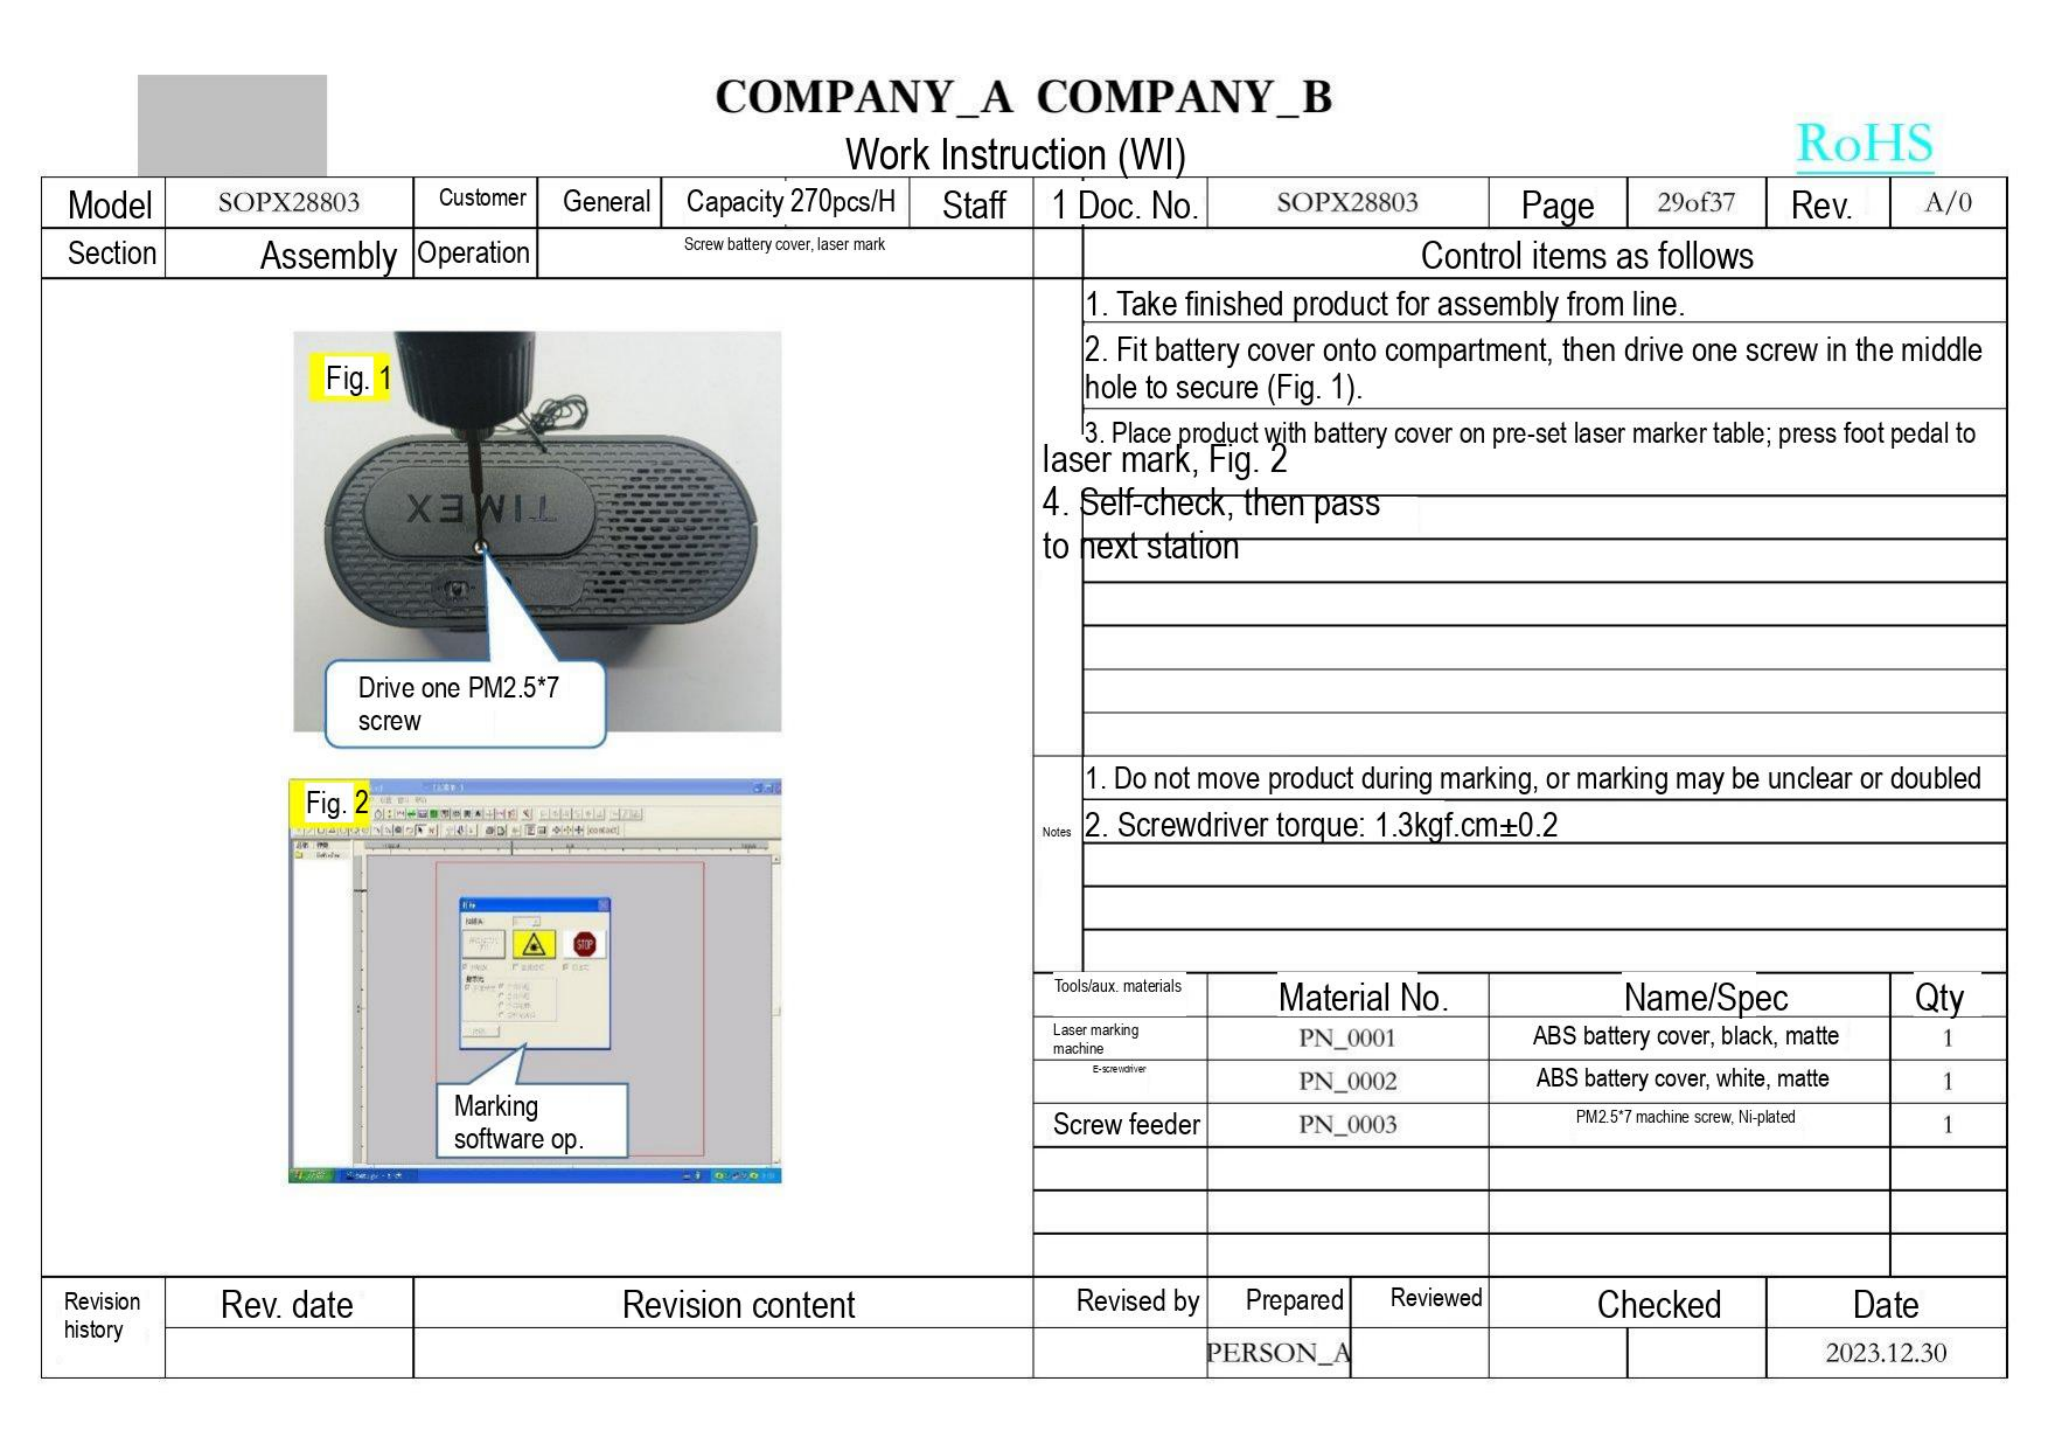# COMPANY_A COMPANY_B
## Work Instruction (WI)
RoHS

| Model | SOPX28803 | Customer | General | Capacity 270pcs/H | Staff | 1 | Doc. No. | SOPX28803 | Page | 29of37 | Rev. | A/0 |
|---|---|---|---|---|---|---|---|---|---|---|---|---|
| Section | Assembly | Operation | Screw battery cover, laser mark | | | | | | | | | |

**Control items as follows**

1. Take finished product for assembly from line.
2. Fit battery cover onto compartment, then drive one screw in the middle hole to secure (Fig. 1).
3. Place product with battery cover on pre-set laser marker table; press foot pedal to laser mark, Fig. 2
4. Self-check, then pass to next station

Fig. 1

Drive one PM2.5*7 screw

Fig. 2

Marking software op.

**Notes**

1. Do not move product during marking, or marking may be unclear or doubled
2. Screwdriver torque: 1.3kgf.cm±0.2

| Tools/aux. materials | Material No. | Name/Spec | Qty |
|---|---|---|---|
| Laser marking machine | PN_0001 | ABS battery cover, black, matte | 1 |
| E-screwdriver | PN_0002 | ABS battery cover, white, matte | 1 |
| Screw feeder | PN_0003 | PM2.5*7 machine screw, Ni-plated | 1 |

| Revision history | Rev. date | Revision content | Revised by | Prepared | Reviewed | Checked | Date |
|---|---|---|---|---|---|---|---|
| | | | | PERSON_A | | | 2023.12.30 |
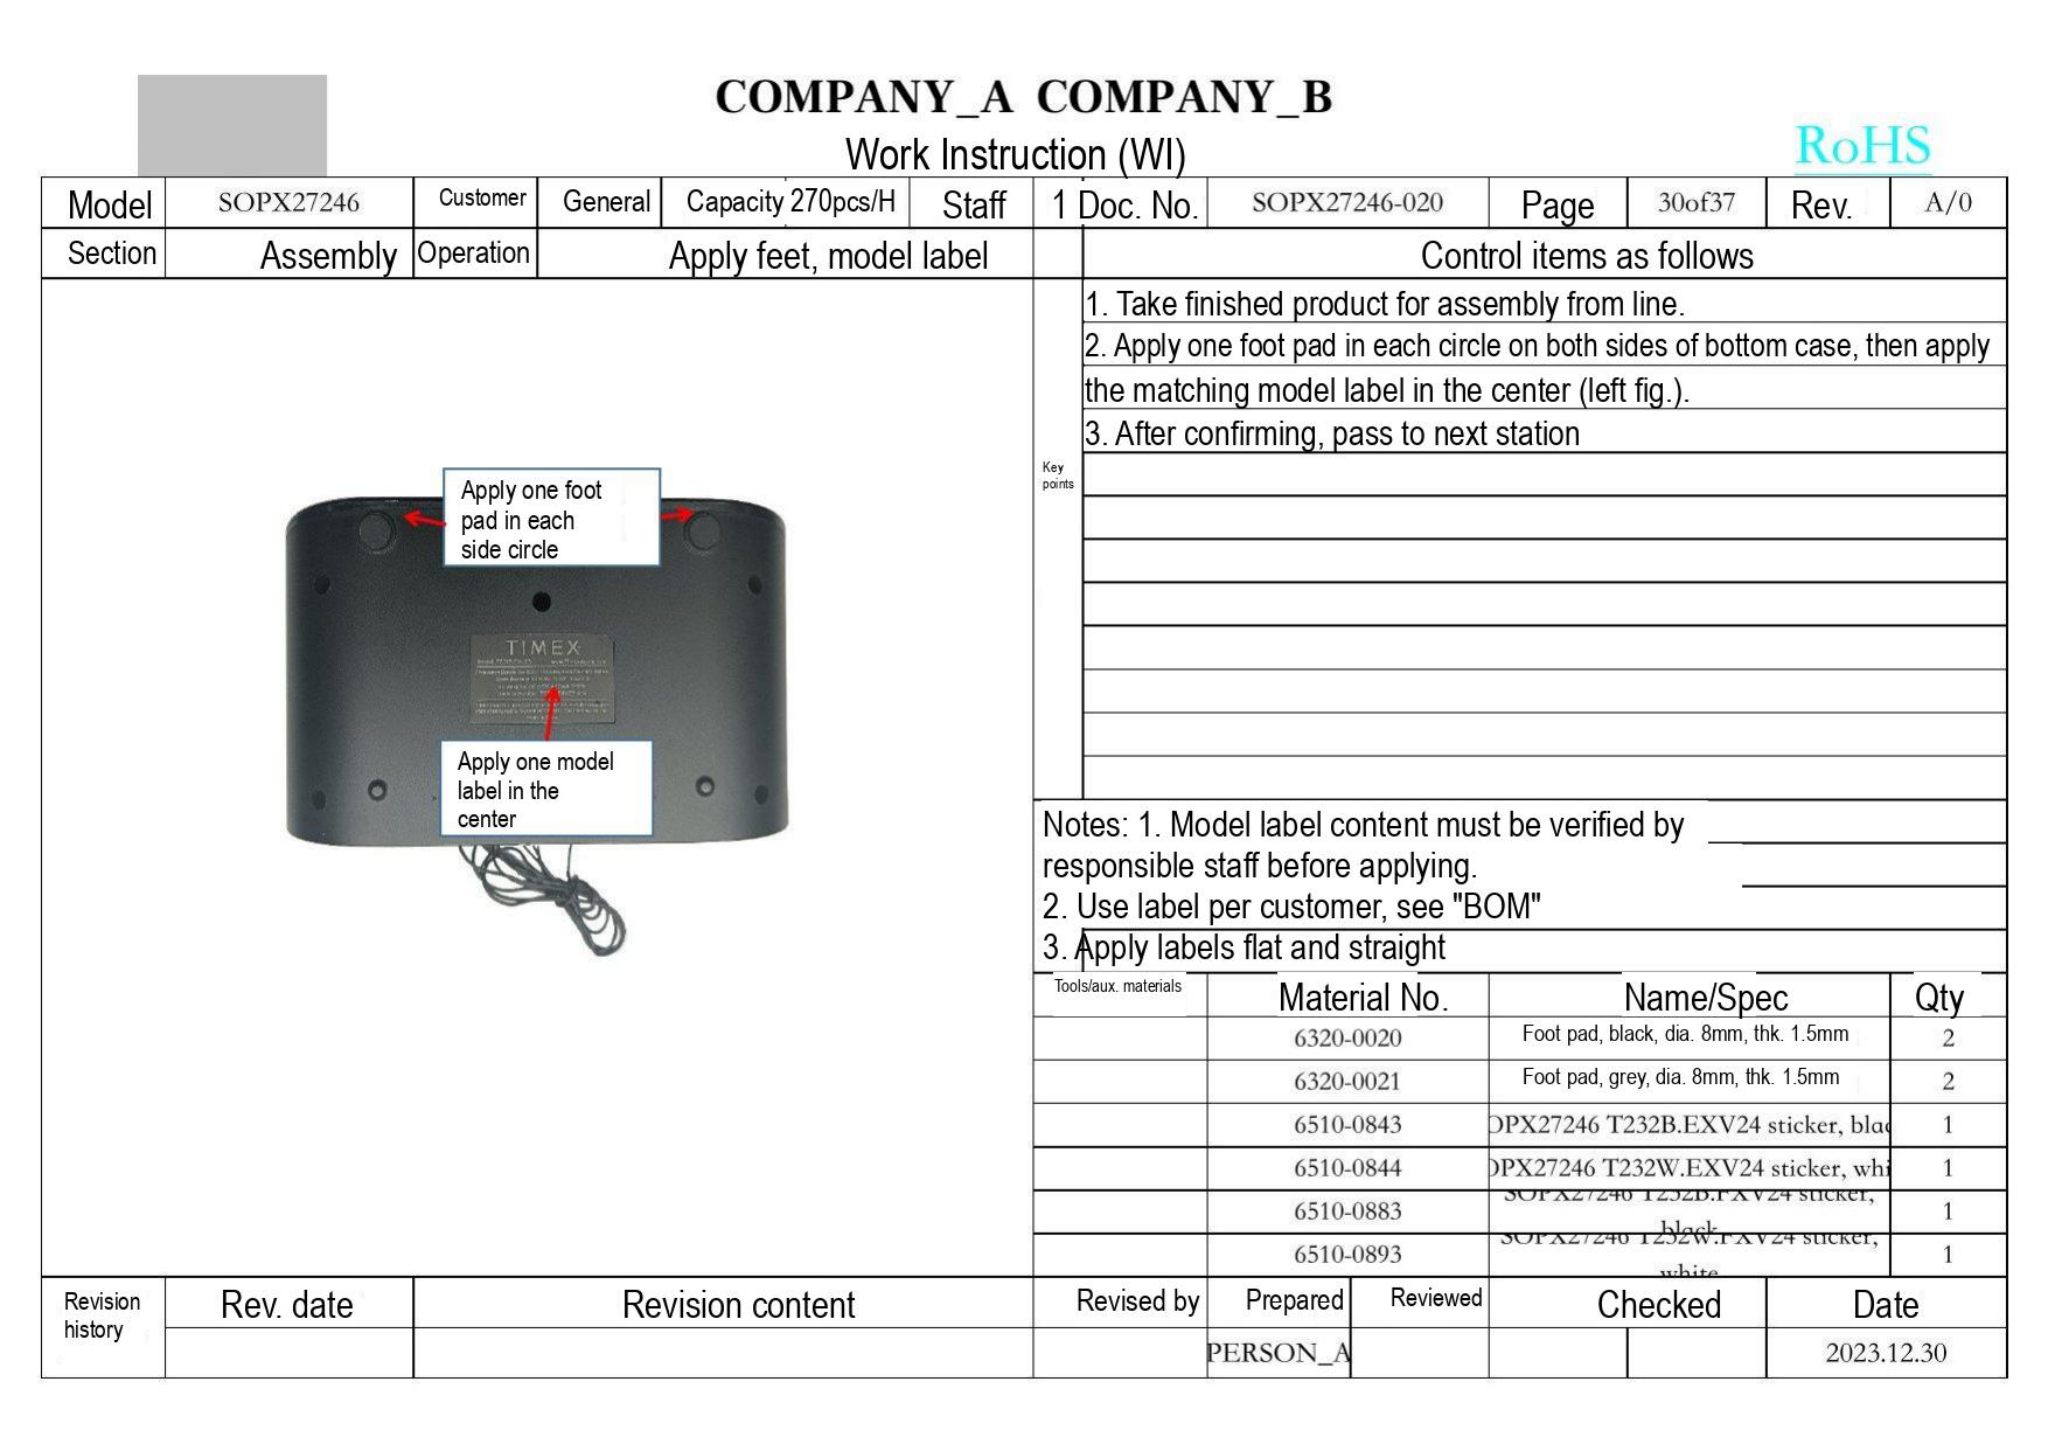COMPANY_A COMPANY_B
Work Instruction (WI)
RoHS

| Model | SOPX27246 | Customer | General | Capacity 270pcs/H | Staff | 1 | Doc. No. | SOPX27246-020 | Page | 30of37 | Rev. | A/0 |
|---|---|---|---|---|---|---|---|---|---|---|---|---|
| Section | Assembly | Operation | Apply feet, model label | | | | | | | | | |

Apply one foot pad in each side circle

TIMEX

Apply one model label in the center

Control items as follows

1. Take finished product for assembly from line.
2. Apply one foot pad in each circle on both sides of bottom case, then apply the matching model label in the center (left fig.).
3. After confirming, pass to next station

Key points

Notes: 1. Model label content must be verified by responsible staff before applying.
2. Use label per customer, see "BOM"
3. Apply labels flat and straight

| Tools/aux. materials | Material No. | Name/Spec | Qty |
|---|---|---|---|
| | 6320-0020 | Foot pad, black, dia. 8mm, thk. 1.5mm | 2 |
| | 6320-0021 | Foot pad, grey, dia. 8mm, thk. 1.5mm | 2 |
| | 6510-0843 | OPX27246 T232B.EXV24 sticker, bla | 1 |
| | 6510-0844 | OPX27246 T232W.EXV24 sticker, whi | 1 |
| | 6510-0883 | SOPX27246 T232B.FXV24 sticker, black | 1 |
| | 6510-0893 | SOPX27246 T232W.FXV24 sticker, white | 1 |

| Revision history | Rev. date | Revision content | Revised by | Prepared | Reviewed | Checked | Date |
|---|---|---|---|---|---|---|---|
| | | | | PERSON_A | | | 2023.12.30 |
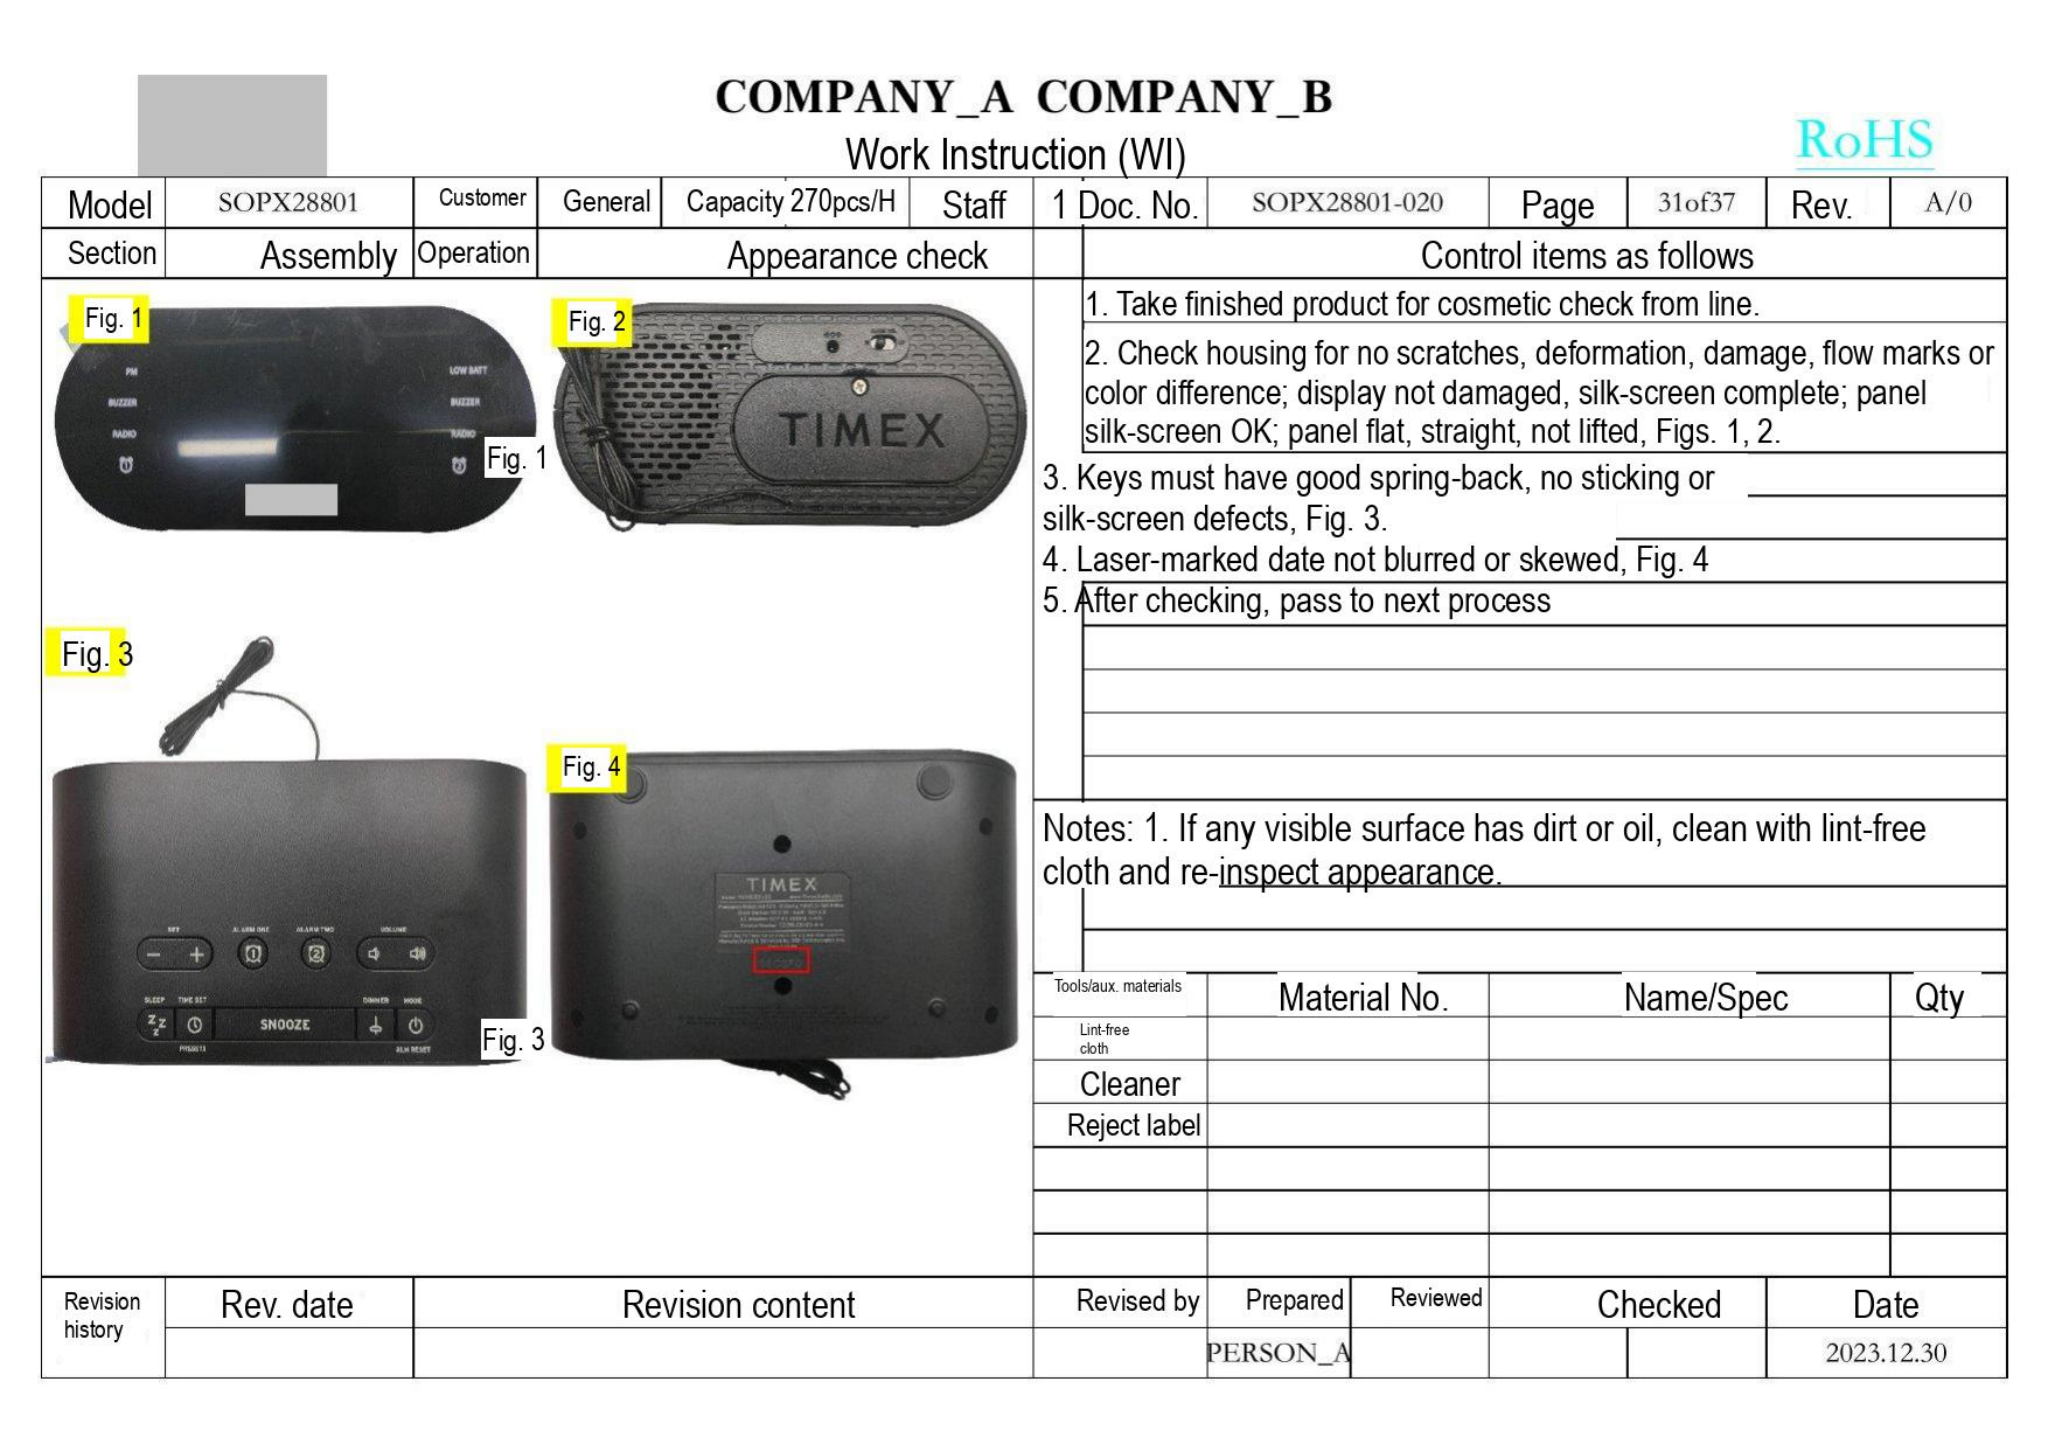COMPANY_A COMPANY_B
Work Instruction (WI)
RoHS

| Model | SOPX28801 | Customer | General | Capacity 270pcs/H | Staff | 1 Doc. No. | SOPX28801-020 | Page | 31of37 | Rev. | A/0 |
|---|---|---|---|---|---|---|---|---|---|---|---|
| Section | Assembly | Operation | Appearance check | | | Control items as follows | | | | | |

Fig. 1
PM
BUZZER
RADIO
LOW BATT
BUZZER
RADIO
Fig. 1

Fig. 2
TIMEX

Fig. 3
SET
ALARM ONE
ALARM TWO
VOLUME
SLEEP
TIME SET
SNOOZE
DIMMER
MODE
PRESETS
ALM RESET
Fig. 3

Fig. 4
TIMEX

Control items as follows
1. Take finished product for cosmetic check from line.
2. Check housing for no scratches, deformation, damage, flow marks or color difference; display not damaged, silk-screen complete; panel silk-screen OK; panel flat, straight, not lifted, Figs. 1, 2.
3. Keys must have good spring-back, no sticking or silk-screen defects, Fig. 3.
4. Laser-marked date not blurred or skewed, Fig. 4
5. After checking, pass to next process

Notes: 1. If any visible surface has dirt or oil, clean with lint-free cloth and re-inspect appearance.

| Tools/aux. materials | Material No. | Name/Spec | Qty |
|---|---|---|---|
| Lint-free cloth | | | |
| Cleaner | | | |
| Reject label | | | |
| | | | |
| | | | |
| | | | |

| Revision history | Rev. date | Revision content | Revised by | Prepared | Reviewed | Checked | Date |
|---|---|---|---|---|---|---|---|
| | | | | PERSON_A | | | 2023.12.30 |
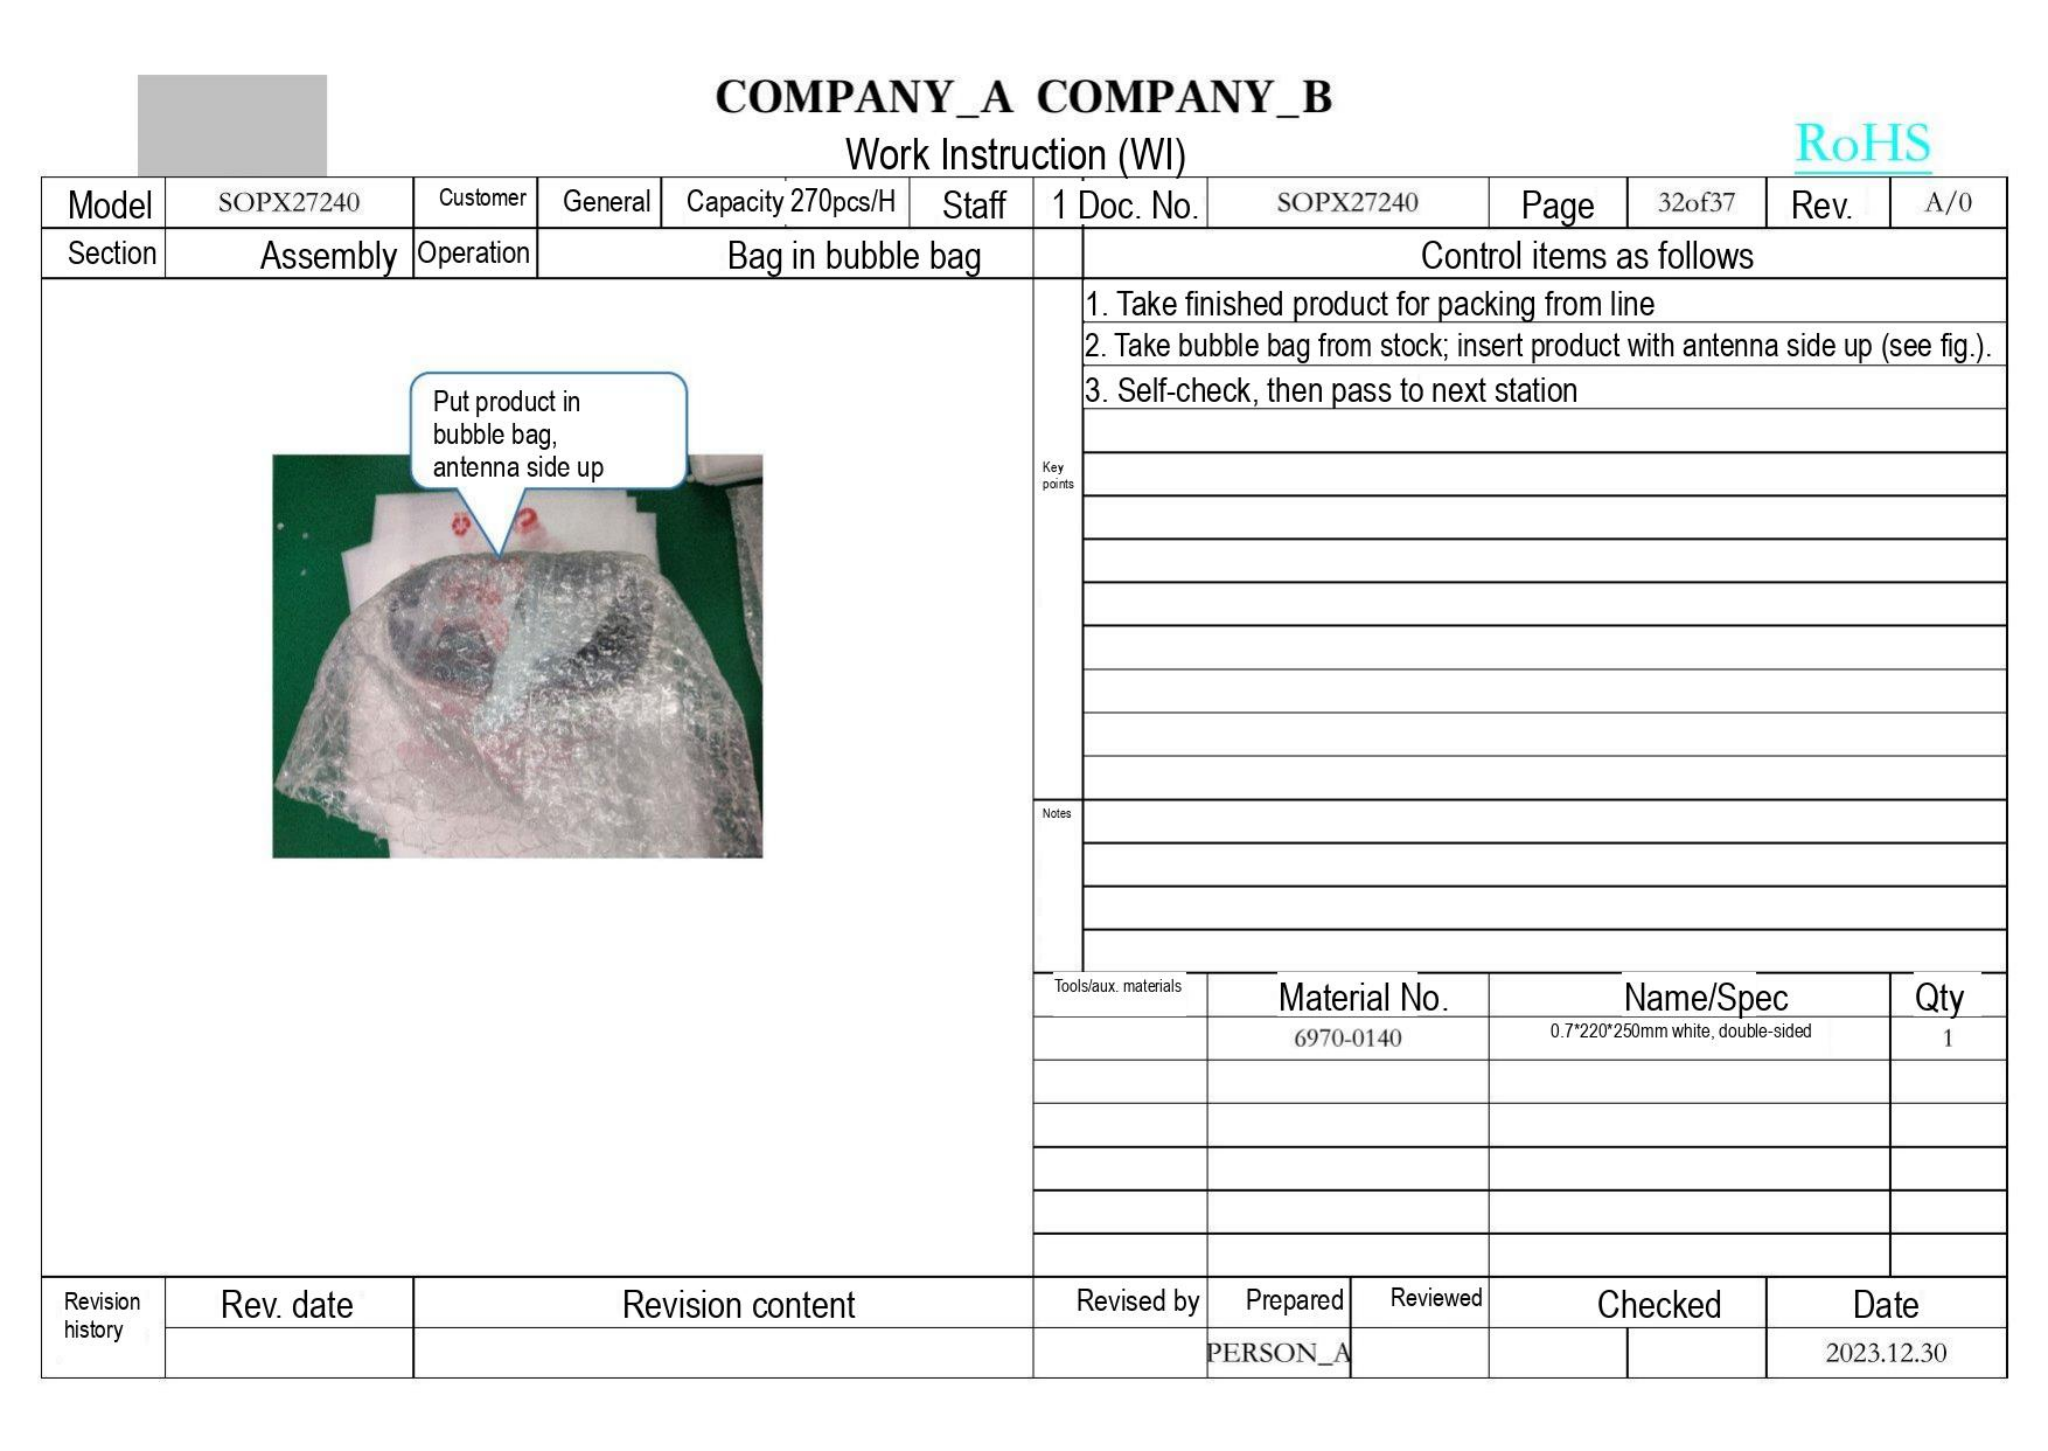COMPANY_A COMPANY_B
Work Instruction (WI)
RoHS

| Model | SOPX27240 | Customer | General | Capacity | 270pcs/H | Staff | 1 | Doc. No. | SOPX27240 | Page | 32of37 | Rev. | A/0 |
|---|---|---|---|---|---|---|---|---|---|---|---|---|---|
| Section | Assembly | Operation | Bag in bubble bag | | | | | Control items as follows | | | | | |

Put product in bubble bag, antenna side up

| | Control items as follows |
|---|---|
| Key points | 1. Take finished product for packing from line |
| | 2. Take bubble bag from stock; insert product with antenna side up (see fig.). |
| | 3. Self-check, then pass to next station |
| Notes | |

| Tools/aux. materials | Material No. | Name/Spec | Qty |
|---|---|---|---|
| | 6970-0140 | 0.7*220*250mm white, double-sided | 1 |

| Revision history | Rev. date | Revision content | Revised by | Prepared | Reviewed | Checked | Date |
|---|---|---|---|---|---|---|---|
| | | | | PERSON_A | | | 2023.12.30 |
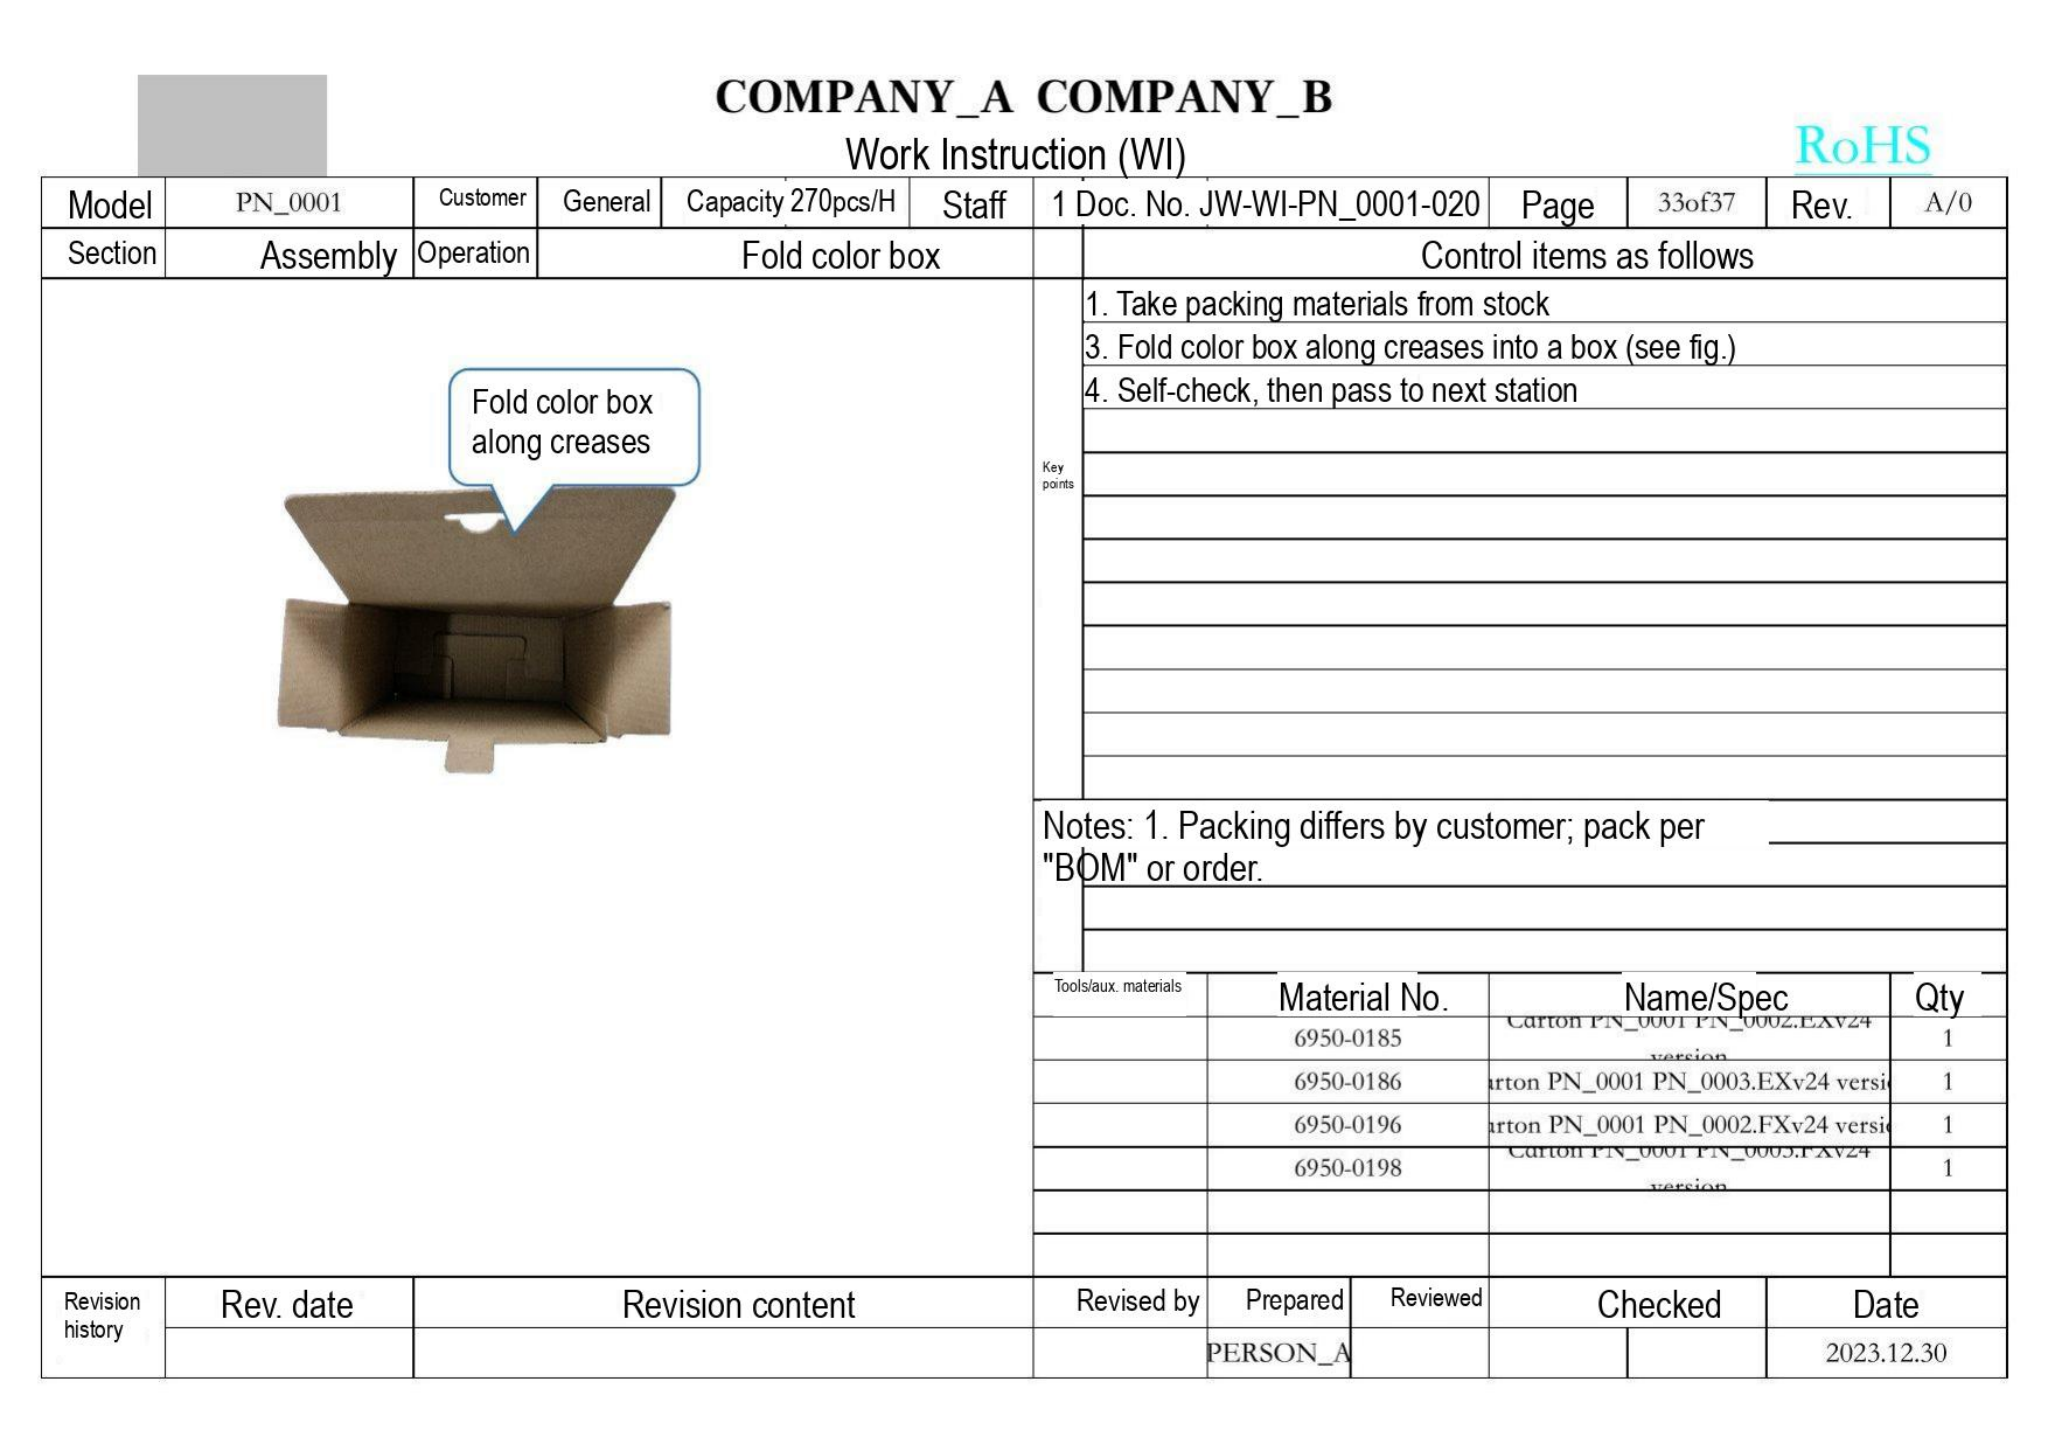COMPANY_A COMPANY_B

Work Instruction (WI)

RoHS

| Model | PN_0001 | Customer | General | Capacity 270pcs/H | Staff | 1 Doc. No. JW-WI-PN_0001-020 | Page | 33of37 | Rev. | A/0 |
|---|---|---|---|---|---|---|---|---|---|---|
| Section | Assembly | Operation | Fold color box | | | | | | | |

Fold color box along creases

Control items as follows

Key points

1. Take packing materials from stock
3. Fold color box along creases into a box (see fig.)
4. Self-check, then pass to next station

Notes: 1. Packing differs by customer; pack per "BOM" or order.

| Tools/aux. materials | Material No. | Name/Spec | Qty |
|---|---|---|---|
| | 6950-0185 | Carton PN_0001 PN_0002.EXv24 version | 1 |
| | 6950-0186 | rton PN_0001 PN_0003.EXv24 versi | 1 |
| | 6950-0196 | rton PN_0001 PN_0002.FXv24 versi | 1 |
| | 6950-0198 | Carton PN_0001 PN_0003.FXv24 version | 1 |
| | | | |
| | | | |

| Revision history | Rev. date | Revision content | Revised by | Prepared | Reviewed | Checked | Date |
|---|---|---|---|---|---|---|---|
| | | | | PERSON_A | | | 2023.12.30 |
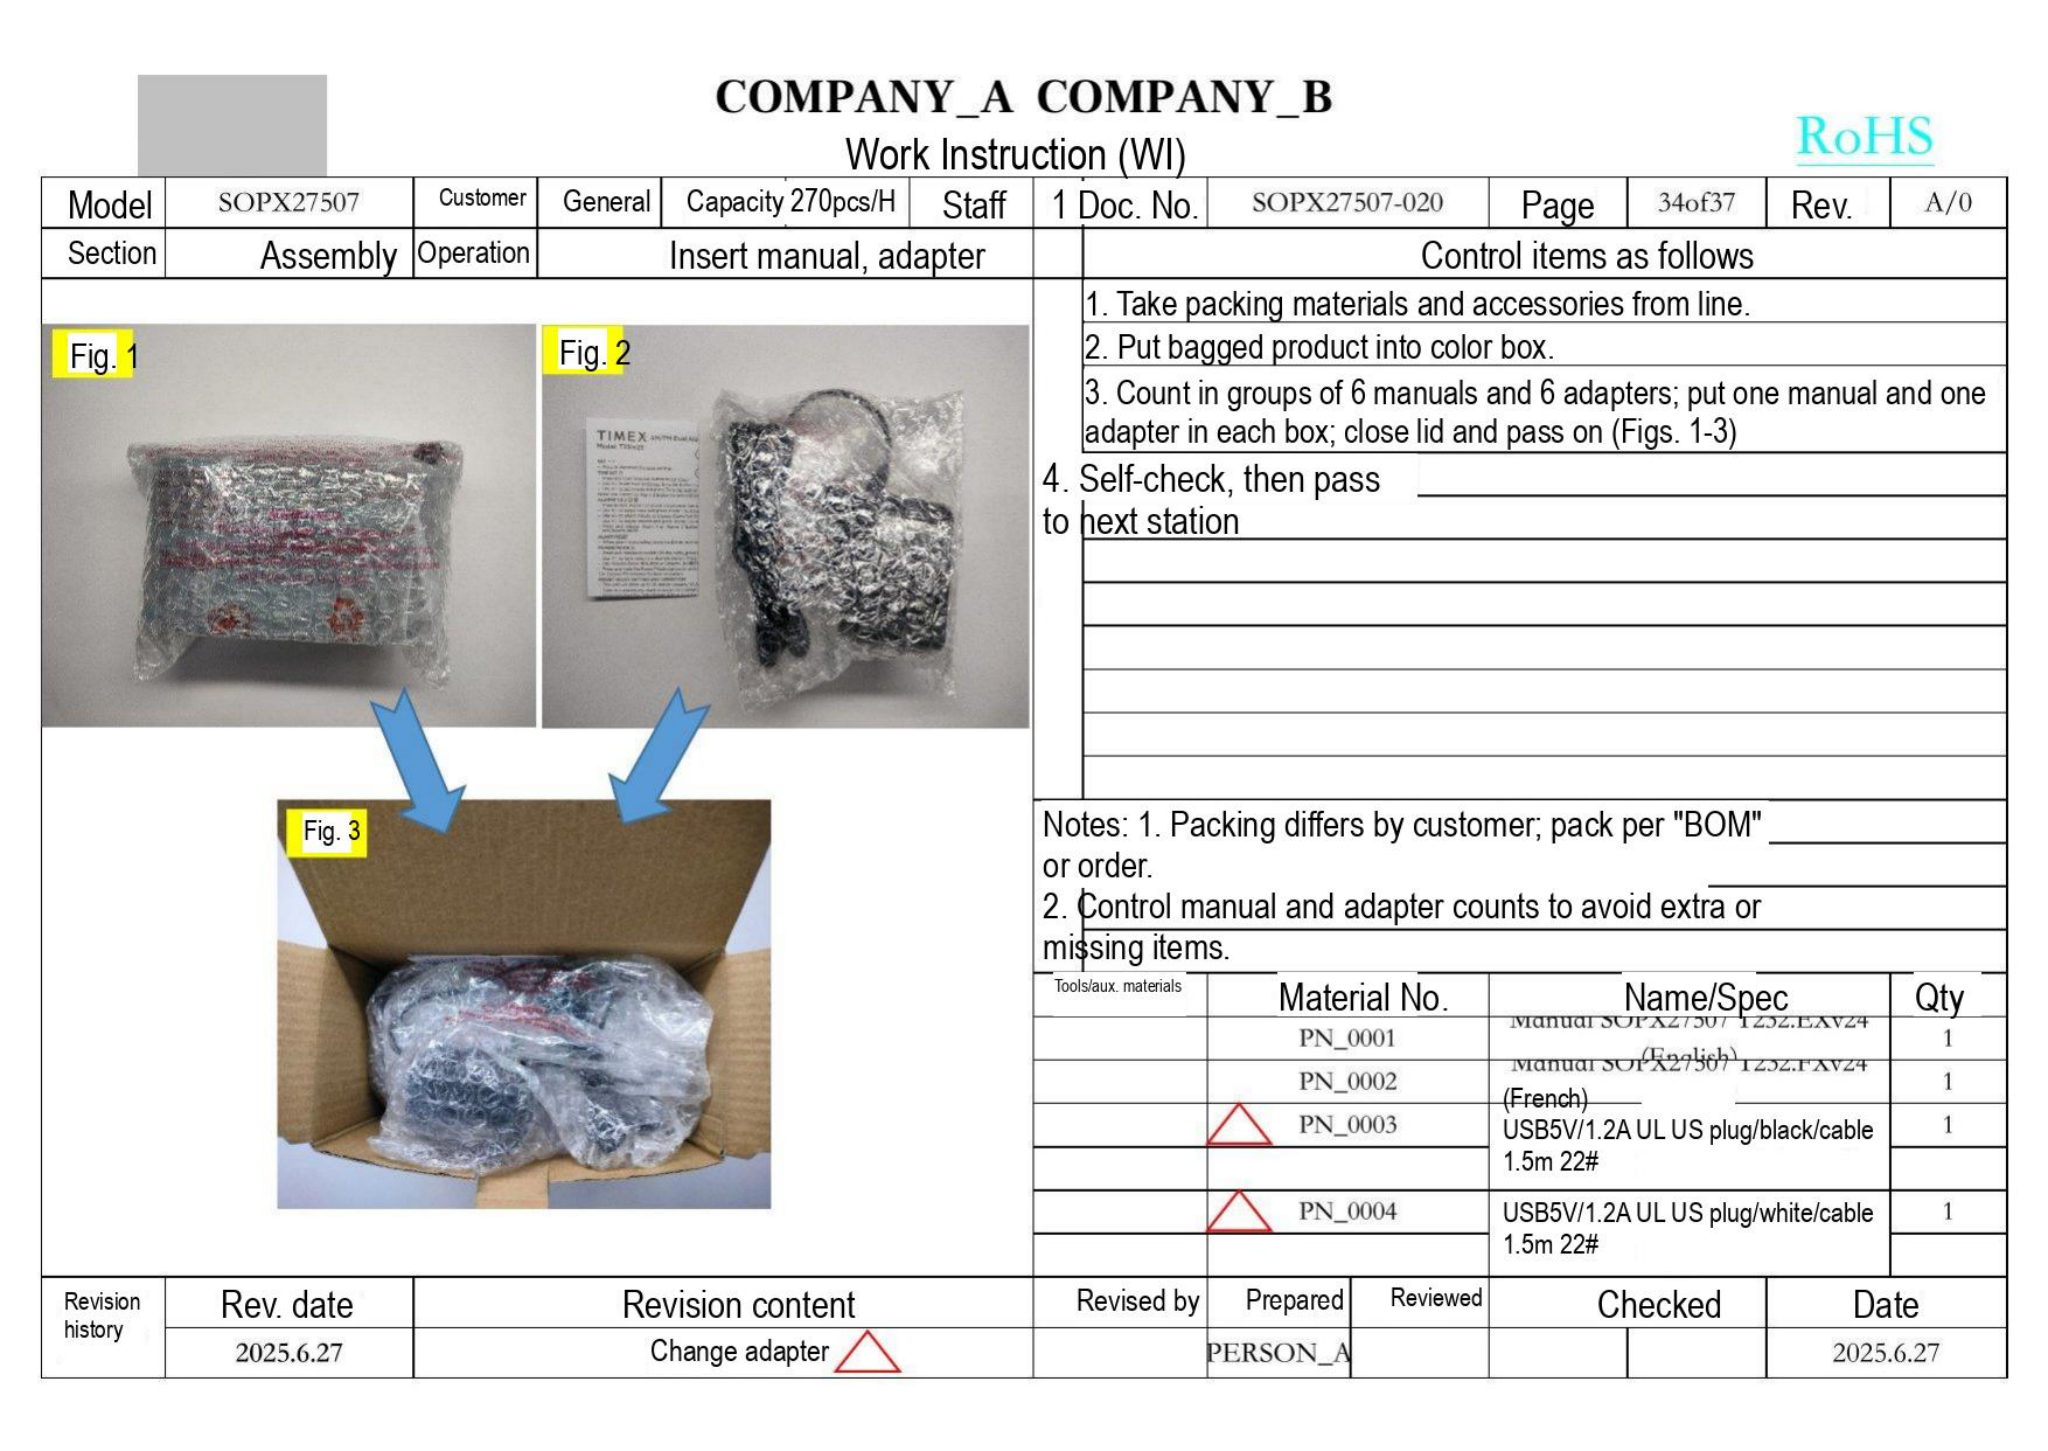COMPANY_A COMPANY_B
Work Instruction (WI)
RoHS

| Model | SOPX27507 | Customer | General | Capacity 270pcs/H | Staff | 1 | Doc. No. | SOPX27507-020 | Page | 34of37 | Rev. | A/0 |
|---|---|---|---|---|---|---|---|---|---|---|---|---|
| Section | Assembly | Operation | Insert manual, adapter | | | | | | | | | |

Fig. 1

Fig. 2
TIMEX

Fig. 3

Control items as follows
1. Take packing materials and accessories from line.
2. Put bagged product into color box.
3. Count in groups of 6 manuals and 6 adapters; put one manual and one adapter in each box; close lid and pass on (Figs. 1-3)
4. Self-check, then pass to next station

Notes: 1. Packing differs by customer; pack per "BOM" or order.
2. Control manual and adapter counts to avoid extra or missing items.

| Tools/aux. materials | Material No. | Name/Spec | Qty |
|---|---|---|---|
| | PN_0001 | Manual SOPX27507 T232.EXV24 (English) | 1 |
| | PN_0002 | Manual SOPX27507 T232.FXV24 (French) | 1 |
| | PN_0003 | USB5V/1.2A UL US plug/black/cable 1.5m 22# | 1 |
| | PN_0004 | USB5V/1.2A UL US plug/white/cable 1.5m 22# | 1 |

| Revision history | Rev. date | Revision content | Revised by | Prepared | Reviewed | Checked | Date |
|---|---|---|---|---|---|---|---|
| | 2025.6.27 | Change adapter | | PERSON_A | | | 2025.6.27 |
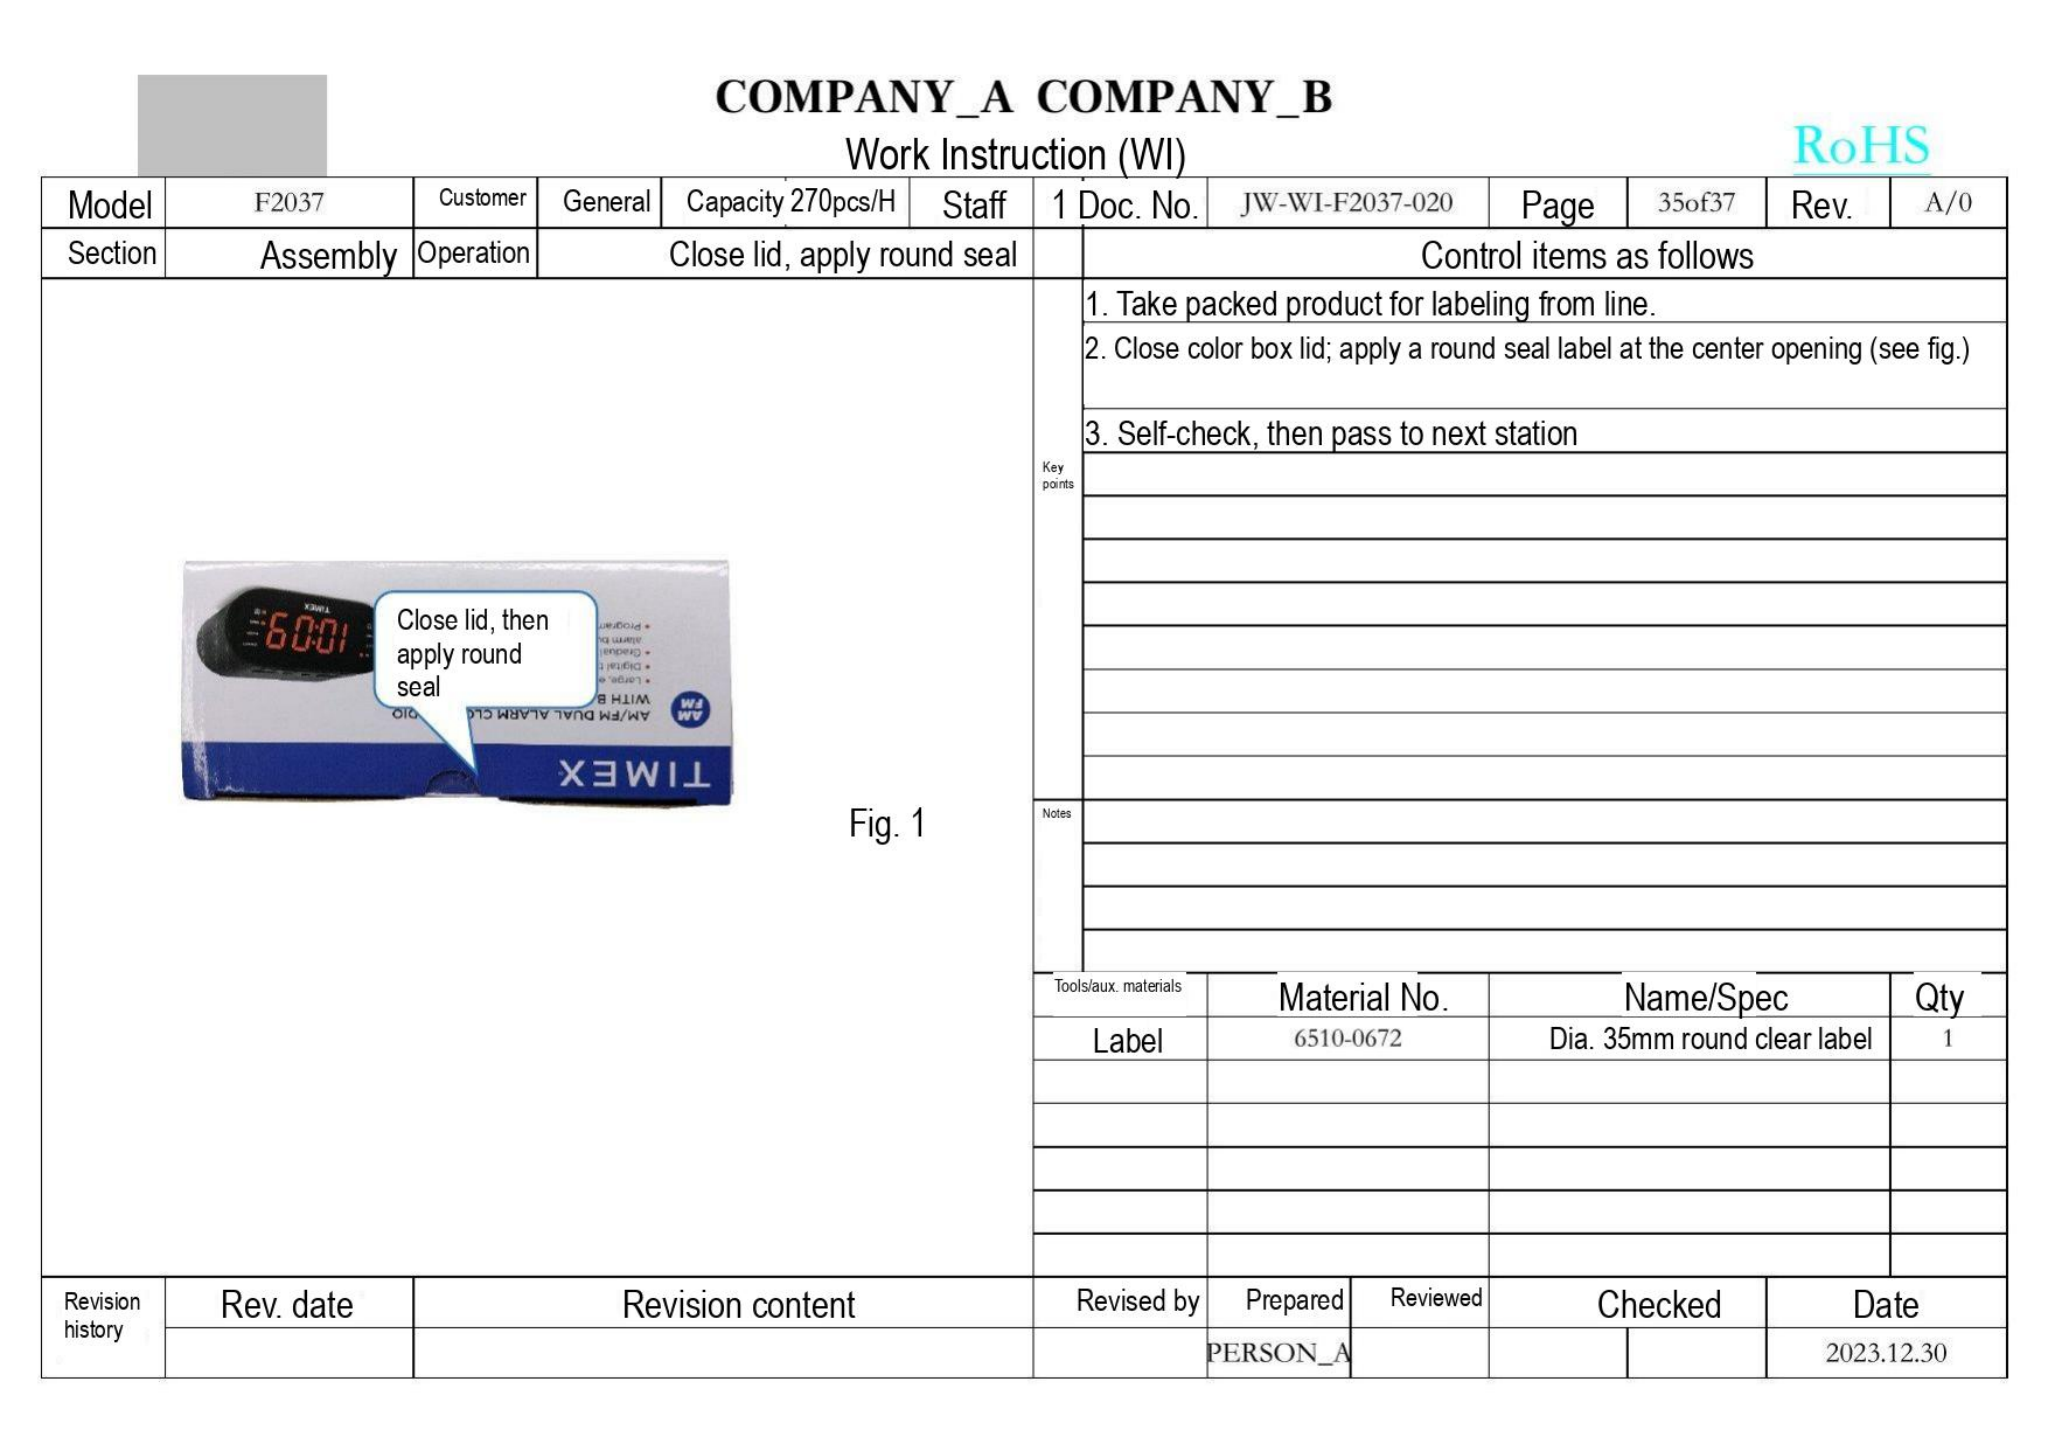COMPANY_A COMPANY_B
Work Instruction (WI)
RoHS

| Model | F2037 | Customer | General | Capacity 270pcs/H | Staff | 1 | Doc. No. | JW-WI-F2037-020 | Page | 35of37 | Rev. | A/0 |
|---|---|---|---|---|---|---|---|---|---|---|---|---|
| Section | Assembly | Operation | Close lid, apply round seal | | | | Control items as follows | | | | | |

Close lid, then apply round seal

AM/FM DUAL ALARM CL

WITH B

TIMEX

Fig. 1

Control items as follows
1. Take packed product for labeling from line.
2. Close color box lid; apply a round seal label at the center opening (see fig.)
3. Self-check, then pass to next station

Key points

Notes

| Tools/aux. materials | Material No. | Name/Spec | Qty |
|---|---|---|---|
| Label | 6510-0672 | Dia. 35mm round clear label | 1 |
| | | | |
| | | | |
| | | | |
| | | | |
| | | | |

| Revision history | Rev. date | Revision content | Revised by | Prepared | Reviewed | Checked | Date |
|---|---|---|---|---|---|---|---|
| | | | | PERSON_A | | | 2023.12.30 |